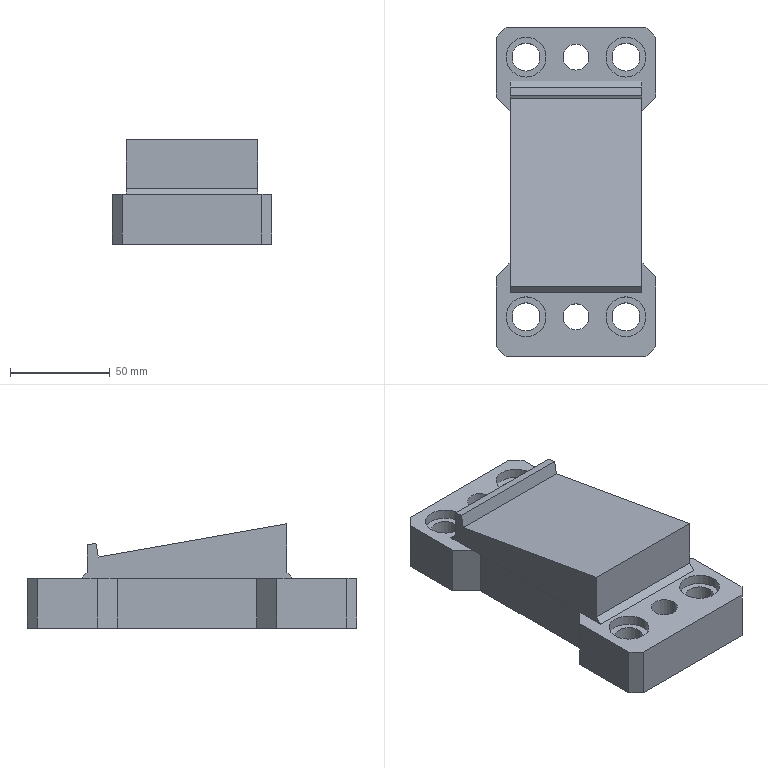Part | NX | features solid 2 | 1 solid | 45 faces | box 80 x 165 x 52.259 mm | volume 388189 mm3 | plane 31 | cylinder 10 | spline 4 | commonest cylinder face diameters 14 x4 20 x4 13 x2
STEP:
#1=CARTESIAN_POINT('',(-445.,-770.,-75.));
#2=VERTEX_POINT('',#1);
#3=CARTESIAN_POINT('',(-375.,-770.,-75.));
#4=VERTEX_POINT('',#3);
#5=CARTESIAN_POINT('',(-410.,-770.,-75.));
#6=DIRECTION('',(1.,0.,0.));
#7=VECTOR('',#6,1000.);
#8=LINE('',#5,#7);
#9=EDGE_CURVE('',#2,#4,#8,.T.);
#10=ORIENTED_EDGE('',*,*,#9,.T.);
#11=CARTESIAN_POINT('',(-370.,-765.,-75.));
#12=VERTEX_POINT('',#11);
#13=CARTESIAN_POINT('',(-351.25,-746.25,-75.));
#14=DIRECTION('',(0.7071,0.7071,0.));
#15=VECTOR('',#14,1000.);
#16=LINE('',#13,#15);
#17=EDGE_CURVE('',#12,#4,#16,.F.);
#18=ORIENTED_EDGE('',*,*,#17,.F.);
#19=CARTESIAN_POINT('',(-370.,-730.,-75.));
#20=VERTEX_POINT('',#19);
#21=CARTESIAN_POINT('',(-370.,-687.5,-75.));
#22=DIRECTION('',(0.,1.,0.));
#23=VECTOR('',#22,1000.);
#24=LINE('',#21,#23);
#25=EDGE_CURVE('',#12,#20,#24,.T.);
#26=ORIENTED_EDGE('',*,*,#25,.T.);
#27=CARTESIAN_POINT('',(-377.,-723.,-75.));
#28=VERTEX_POINT('',#27);
#29=CARTESIAN_POINT('',(-370.,-730.,-75.));
#30=DIRECTION('',(-0.7071,0.7071,0.));
#31=VECTOR('',#30,1000.);
#32=LINE('',#29,#31);
#33=EDGE_CURVE('',#20,#28,#32,.T.);
#34=ORIENTED_EDGE('',*,*,#33,.T.);
#35=CARTESIAN_POINT('',(-377.,-738.,-75.));
#36=VERTEX_POINT('',#35);
#37=CARTESIAN_POINT('',(-377.,-735.,-75.));
#38=DIRECTION('',(0.,1.,0.));
#39=VECTOR('',#38,1000.);
#40=LINE('',#37,#39);
#41=EDGE_CURVE('',#36,#28,#40,.T.);
#42=ORIENTED_EDGE('',*,*,#41,.F.);
#43=CARTESIAN_POINT('',(-443.,-738.,-75.));
#44=VERTEX_POINT('',#43);
#45=CARTESIAN_POINT('',(-410.,-738.,-75.));
#46=DIRECTION('',(1.,0.,0.));
#47=VECTOR('',#46,1000.);
#48=LINE('',#45,#47);
#49=EDGE_CURVE('',#44,#36,#48,.T.);
#50=ORIENTED_EDGE('',*,*,#49,.F.);
#51=CARTESIAN_POINT('',(-443.,-723.,-75.));
#52=VERTEX_POINT('',#51);
#53=CARTESIAN_POINT('',(-443.,-735.,-75.));
#54=DIRECTION('',(0.,1.,0.));
#55=VECTOR('',#54,1000.);
#56=LINE('',#53,#55);
#57=EDGE_CURVE('',#44,#52,#56,.T.);
#58=ORIENTED_EDGE('',*,*,#57,.T.);
#59=CARTESIAN_POINT('',(-450.,-730.,-75.));
#60=VERTEX_POINT('',#59);
#61=CARTESIAN_POINT('',(-440.,-720.,-75.));
#62=DIRECTION('',(-0.7071,-0.7071,0.));
#63=VECTOR('',#62,1000.);
#64=LINE('',#61,#63);
#65=EDGE_CURVE('',#52,#60,#64,.T.);
#66=ORIENTED_EDGE('',*,*,#65,.T.);
#67=CARTESIAN_POINT('',(-450.,-765.,-75.));
#68=VERTEX_POINT('',#67);
#69=CARTESIAN_POINT('',(-450.,-687.5,-75.));
#70=DIRECTION('',(0.,-1.,0.));
#71=VECTOR('',#70,1000.);
#72=LINE('',#69,#71);
#73=EDGE_CURVE('',#60,#68,#72,.T.);
#74=ORIENTED_EDGE('',*,*,#73,.T.);
#75=CARTESIAN_POINT('',(-468.75,-746.25,-75.));
#76=DIRECTION('',(0.7071,-0.7071,0.));
#77=VECTOR('',#76,1000.);
#78=LINE('',#75,#77);
#79=EDGE_CURVE('',#2,#68,#78,.F.);
#80=ORIENTED_EDGE('',*,*,#79,.F.);
#81=EDGE_LOOP('',(#10,#18,#26,#34,#42,#50,#58,#66,#74,#80));
#82=FACE_BOUND('',#81,.T.);
#83=CARTESIAN_POINT('',(-385.,-740.,-75.));
#84=VERTEX_POINT('',#83);
#85=CARTESIAN_POINT('',(-385.,-750.,-75.));
#86=DIRECTION('',(0.,0.,-1.));
#87=DIRECTION('',(0.,1.,0.));
#88=AXIS2_PLACEMENT_3D('',#85,#86,#87);
#89=CIRCLE('',#88,10.);
#90=EDGE_CURVE('',#84,#84,#89,.T.);
#91=ORIENTED_EDGE('',*,*,#90,.T.);
#92=EDGE_LOOP('',(#91));
#93=FACE_BOUND('',#92,.T.);
#94=CARTESIAN_POINT('',(-410.,-743.5,-75.));
#95=VERTEX_POINT('',#94);
#96=CARTESIAN_POINT('',(-410.,-750.,-75.));
#97=DIRECTION('',(0.,0.,-1.));
#98=DIRECTION('',(0.,1.,0.));
#99=AXIS2_PLACEMENT_3D('',#96,#97,#98);
#100=CIRCLE('',#99,6.5);
#101=EDGE_CURVE('',#95,#95,#100,.T.);
#102=ORIENTED_EDGE('',*,*,#101,.T.);
#103=EDGE_LOOP('',(#102));
#104=FACE_BOUND('',#103,.T.);
#105=CARTESIAN_POINT('',(-435.,-740.,-75.));
#106=VERTEX_POINT('',#105);
#107=CARTESIAN_POINT('',(-435.,-750.,-75.));
#108=DIRECTION('',(0.,0.,-1.));
#109=DIRECTION('',(0.,1.,0.));
#110=AXIS2_PLACEMENT_3D('',#107,#108,#109);
#111=CIRCLE('',#110,10.);
#112=EDGE_CURVE('',#106,#106,#111,.T.);
#113=ORIENTED_EDGE('',*,*,#112,.T.);
#114=EDGE_LOOP('',(#113));
#115=FACE_BOUND('',#114,.T.);
#116=CARTESIAN_POINT('',(-410.,-687.5,-75.));
#117=DIRECTION('',(0.,0.,1.));
#118=DIRECTION('',(0.,1.,0.));
#119=AXIS2_PLACEMENT_3D('',#116,#117,#118);
#120=PLANE('',#119);
#121=ADVANCED_FACE('',(#82,#93,#104,#115),#120,.T.);
#122=CARTESIAN_POINT('',(-375.,-605.,-75.));
#123=VERTEX_POINT('',#122);
#124=CARTESIAN_POINT('',(-445.,-605.,-75.));
#125=VERTEX_POINT('',#124);
#126=CARTESIAN_POINT('',(-410.,-605.,-75.));
#127=DIRECTION('',(-1.,0.,0.));
#128=VECTOR('',#127,1000.);
#129=LINE('',#126,#128);
#130=EDGE_CURVE('',#123,#125,#129,.T.);
#131=ORIENTED_EDGE('',*,*,#130,.T.);
#132=CARTESIAN_POINT('',(-450.,-610.,-75.));
#133=VERTEX_POINT('',#132);
#134=CARTESIAN_POINT('',(-468.75,-628.75,-75.));
#135=DIRECTION('',(-0.7071,-0.7071,0.));
#136=VECTOR('',#135,1000.);
#137=LINE('',#134,#136);
#138=EDGE_CURVE('',#133,#125,#137,.F.);
#139=ORIENTED_EDGE('',*,*,#138,.F.);
#140=CARTESIAN_POINT('',(-450.,-640.,-75.));
#141=VERTEX_POINT('',#140);
#142=CARTESIAN_POINT('',(-450.,-687.5,-75.));
#143=DIRECTION('',(0.,-1.,0.));
#144=VECTOR('',#143,1000.);
#145=LINE('',#142,#144);
#146=EDGE_CURVE('',#133,#141,#145,.T.);
#147=ORIENTED_EDGE('',*,*,#146,.T.);
#148=CARTESIAN_POINT('',(-443.,-647.,-75.));
#149=VERTEX_POINT('',#148);
#150=CARTESIAN_POINT('',(-440.,-650.,-75.));
#151=DIRECTION('',(-0.7071,0.7071,0.));
#152=VECTOR('',#151,1000.);
#153=LINE('',#150,#152);
#154=EDGE_CURVE('',#149,#141,#153,.T.);
#155=ORIENTED_EDGE('',*,*,#154,.F.);
#156=CARTESIAN_POINT('',(-443.,-632.,-75.));
#157=VERTEX_POINT('',#156);
#158=CARTESIAN_POINT('',(-443.,-735.,-75.));
#159=DIRECTION('',(0.,1.,0.));
#160=VECTOR('',#159,1000.);
#161=LINE('',#158,#160);
#162=EDGE_CURVE('',#149,#157,#161,.T.);
#163=ORIENTED_EDGE('',*,*,#162,.T.);
#164=CARTESIAN_POINT('',(-377.,-632.,-75.));
#165=VERTEX_POINT('',#164);
#166=CARTESIAN_POINT('',(-443.,-632.,-75.));
#167=DIRECTION('',(-1.,0.,0.));
#168=VECTOR('',#167,1000.);
#169=LINE('',#166,#168);
#170=EDGE_CURVE('',#165,#157,#169,.T.);
#171=ORIENTED_EDGE('',*,*,#170,.F.);
#172=CARTESIAN_POINT('',(-377.,-647.,-75.));
#173=VERTEX_POINT('',#172);
#174=CARTESIAN_POINT('',(-377.,-735.,-75.));
#175=DIRECTION('',(0.,1.,0.));
#176=VECTOR('',#175,1000.);
#177=LINE('',#174,#176);
#178=EDGE_CURVE('',#173,#165,#177,.T.);
#179=ORIENTED_EDGE('',*,*,#178,.F.);
#180=CARTESIAN_POINT('',(-370.,-640.,-75.));
#181=VERTEX_POINT('',#180);
#182=CARTESIAN_POINT('',(-370.,-640.,-75.));
#183=DIRECTION('',(-0.7071,-0.7071,0.));
#184=VECTOR('',#183,1000.);
#185=LINE('',#182,#184);
#186=EDGE_CURVE('',#181,#173,#185,.T.);
#187=ORIENTED_EDGE('',*,*,#186,.F.);
#188=CARTESIAN_POINT('',(-370.,-610.,-75.));
#189=VERTEX_POINT('',#188);
#190=CARTESIAN_POINT('',(-370.,-687.5,-75.));
#191=DIRECTION('',(0.,1.,0.));
#192=VECTOR('',#191,1000.);
#193=LINE('',#190,#192);
#194=EDGE_CURVE('',#181,#189,#193,.T.);
#195=ORIENTED_EDGE('',*,*,#194,.T.);
#196=CARTESIAN_POINT('',(-351.25,-628.75,-75.));
#197=DIRECTION('',(-0.7071,0.7071,0.));
#198=VECTOR('',#197,1000.);
#199=LINE('',#196,#198);
#200=EDGE_CURVE('',#123,#189,#199,.F.);
#201=ORIENTED_EDGE('',*,*,#200,.F.);
#202=EDGE_LOOP('',(#131,#139,#147,#155,#163,#171,#179,#187,#195,#201));
#203=FACE_BOUND('',#202,.T.);
#204=CARTESIAN_POINT('',(-385.,-610.,-75.));
#205=VERTEX_POINT('',#204);
#206=CARTESIAN_POINT('',(-385.,-620.,-75.));
#207=DIRECTION('',(0.,0.,-1.));
#208=DIRECTION('',(0.,1.,0.));
#209=AXIS2_PLACEMENT_3D('',#206,#207,#208);
#210=CIRCLE('',#209,10.);
#211=EDGE_CURVE('',#205,#205,#210,.T.);
#212=ORIENTED_EDGE('',*,*,#211,.T.);
#213=EDGE_LOOP('',(#212));
#214=FACE_BOUND('',#213,.T.);
#215=CARTESIAN_POINT('',(-410.,-613.5,-75.));
#216=VERTEX_POINT('',#215);
#217=CARTESIAN_POINT('',(-410.,-620.,-75.));
#218=DIRECTION('',(0.,0.,-1.));
#219=DIRECTION('',(0.,1.,0.));
#220=AXIS2_PLACEMENT_3D('',#217,#218,#219);
#221=CIRCLE('',#220,6.5);
#222=EDGE_CURVE('',#216,#216,#221,.T.);
#223=ORIENTED_EDGE('',*,*,#222,.T.);
#224=EDGE_LOOP('',(#223));
#225=FACE_BOUND('',#224,.T.);
#226=CARTESIAN_POINT('',(-435.,-610.,-75.));
#227=VERTEX_POINT('',#226);
#228=CARTESIAN_POINT('',(-435.,-620.,-75.));
#229=DIRECTION('',(0.,0.,-1.));
#230=DIRECTION('',(0.,1.,0.));
#231=AXIS2_PLACEMENT_3D('',#228,#229,#230);
#232=CIRCLE('',#231,10.);
#233=EDGE_CURVE('',#227,#227,#232,.T.);
#234=ORIENTED_EDGE('',*,*,#233,.T.);
#235=EDGE_LOOP('',(#234));
#236=FACE_BOUND('',#235,.T.);
#237=CARTESIAN_POINT('',(-410.,-687.5,-75.));
#238=DIRECTION('',(0.,0.,1.));
#239=DIRECTION('',(0.,1.,0.));
#240=AXIS2_PLACEMENT_3D('',#237,#238,#239);
#241=PLANE('',#240);
#242=ADVANCED_FACE('',(#203,#214,#225,#236),#241,.T.);
#243=CARTESIAN_POINT('',(-385.,-743.,-100.));
#244=VERTEX_POINT('',#243);
#245=CARTESIAN_POINT('',(-385.,-750.,-100.));
#246=DIRECTION('',(0.,0.,-1.));
#247=DIRECTION('',(0.,1.,0.));
#248=AXIS2_PLACEMENT_3D('',#245,#246,#247);
#249=CIRCLE('',#248,7.);
#250=EDGE_CURVE('',#244,#244,#249,.T.);
#251=ORIENTED_EDGE('',*,*,#250,.T.);
#252=EDGE_LOOP('',(#251));
#253=FACE_BOUND('',#252,.T.);
#254=CARTESIAN_POINT('',(-385.,-757.,-80.));
#255=VERTEX_POINT('',#254);
#256=CARTESIAN_POINT('',(-385.,-750.,-80.));
#257=DIRECTION('',(0.,0.,-1.));
#258=DIRECTION('',(0.,-1.,0.));
#259=AXIS2_PLACEMENT_3D('',#256,#257,#258);
#260=CIRCLE('',#259,7.);
#261=EDGE_CURVE('',#255,#255,#260,.T.);
#262=ORIENTED_EDGE('',*,*,#261,.F.);
#263=EDGE_LOOP('',(#262));
#264=FACE_BOUND('',#263,.T.);
#265=CARTESIAN_POINT('',(-385.,-750.,-75.));
#266=DIRECTION('',(0.,0.,-1.));
#267=DIRECTION('',(1.,0.,0.));
#268=AXIS2_PLACEMENT_3D('',#265,#266,#267);
#269=CYLINDRICAL_SURFACE('',#268,7.);
#270=ADVANCED_FACE('',(#253,#264),#269,.F.);
#271=CARTESIAN_POINT('',(-435.,-743.,-100.));
#272=VERTEX_POINT('',#271);
#273=CARTESIAN_POINT('',(-435.,-750.,-100.));
#274=DIRECTION('',(0.,0.,-1.));
#275=DIRECTION('',(0.,1.,0.));
#276=AXIS2_PLACEMENT_3D('',#273,#274,#275);
#277=CIRCLE('',#276,7.);
#278=EDGE_CURVE('',#272,#272,#277,.T.);
#279=ORIENTED_EDGE('',*,*,#278,.T.);
#280=EDGE_LOOP('',(#279));
#281=FACE_BOUND('',#280,.T.);
#282=CARTESIAN_POINT('',(-435.,-757.,-80.));
#283=VERTEX_POINT('',#282);
#284=CARTESIAN_POINT('',(-435.,-750.,-80.));
#285=DIRECTION('',(0.,0.,-1.));
#286=DIRECTION('',(0.,-1.,0.));
#287=AXIS2_PLACEMENT_3D('',#284,#285,#286);
#288=CIRCLE('',#287,7.);
#289=EDGE_CURVE('',#283,#283,#288,.T.);
#290=ORIENTED_EDGE('',*,*,#289,.F.);
#291=EDGE_LOOP('',(#290));
#292=FACE_BOUND('',#291,.T.);
#293=CARTESIAN_POINT('',(-435.,-750.,-75.));
#294=DIRECTION('',(0.,0.,-1.));
#295=DIRECTION('',(1.,0.,0.));
#296=AXIS2_PLACEMENT_3D('',#293,#294,#295);
#297=CYLINDRICAL_SURFACE('',#296,7.);
#298=ADVANCED_FACE('',(#281,#292),#297,.F.);
#299=CARTESIAN_POINT('',(-435.,-613.,-100.));
#300=VERTEX_POINT('',#299);
#301=CARTESIAN_POINT('',(-435.,-620.,-100.));
#302=DIRECTION('',(0.,0.,-1.));
#303=DIRECTION('',(0.,1.,0.));
#304=AXIS2_PLACEMENT_3D('',#301,#302,#303);
#305=CIRCLE('',#304,7.);
#306=EDGE_CURVE('',#300,#300,#305,.T.);
#307=ORIENTED_EDGE('',*,*,#306,.T.);
#308=EDGE_LOOP('',(#307));
#309=FACE_BOUND('',#308,.T.);
#310=CARTESIAN_POINT('',(-435.,-627.,-80.));
#311=VERTEX_POINT('',#310);
#312=CARTESIAN_POINT('',(-435.,-620.,-80.));
#313=DIRECTION('',(0.,0.,-1.));
#314=DIRECTION('',(0.,-1.,0.));
#315=AXIS2_PLACEMENT_3D('',#312,#313,#314);
#316=CIRCLE('',#315,7.);
#317=EDGE_CURVE('',#311,#311,#316,.T.);
#318=ORIENTED_EDGE('',*,*,#317,.F.);
#319=EDGE_LOOP('',(#318));
#320=FACE_BOUND('',#319,.T.);
#321=CARTESIAN_POINT('',(-435.,-620.,-75.));
#322=DIRECTION('',(0.,0.,-1.));
#323=DIRECTION('',(1.,0.,0.));
#324=AXIS2_PLACEMENT_3D('',#321,#322,#323);
#325=CYLINDRICAL_SURFACE('',#324,7.);
#326=ADVANCED_FACE('',(#309,#320),#325,.F.);
#327=CARTESIAN_POINT('',(-385.,-613.,-100.));
#328=VERTEX_POINT('',#327);
#329=CARTESIAN_POINT('',(-385.,-620.,-100.));
#330=DIRECTION('',(0.,0.,-1.));
#331=DIRECTION('',(0.,1.,0.));
#332=AXIS2_PLACEMENT_3D('',#329,#330,#331);
#333=CIRCLE('',#332,7.);
#334=EDGE_CURVE('',#328,#328,#333,.T.);
#335=ORIENTED_EDGE('',*,*,#334,.T.);
#336=EDGE_LOOP('',(#335));
#337=FACE_BOUND('',#336,.T.);
#338=CARTESIAN_POINT('',(-385.,-627.,-80.));
#339=VERTEX_POINT('',#338);
#340=CARTESIAN_POINT('',(-385.,-620.,-80.));
#341=DIRECTION('',(0.,0.,-1.));
#342=DIRECTION('',(0.,-1.,0.));
#343=AXIS2_PLACEMENT_3D('',#340,#341,#342);
#344=CIRCLE('',#343,7.);
#345=EDGE_CURVE('',#339,#339,#344,.T.);
#346=ORIENTED_EDGE('',*,*,#345,.F.);
#347=EDGE_LOOP('',(#346));
#348=FACE_BOUND('',#347,.T.);
#349=CARTESIAN_POINT('',(-385.,-620.,-75.));
#350=DIRECTION('',(0.,0.,-1.));
#351=DIRECTION('',(1.,0.,0.));
#352=AXIS2_PLACEMENT_3D('',#349,#350,#351);
#353=CYLINDRICAL_SURFACE('',#352,7.);
#354=ADVANCED_FACE('',(#337,#348),#353,.F.);
#355=CARTESIAN_POINT('',(-410.,-743.5,-100.));
#356=VERTEX_POINT('',#355);
#357=CARTESIAN_POINT('',(-410.,-750.,-100.));
#358=DIRECTION('',(0.,0.,-1.));
#359=DIRECTION('',(0.,1.,0.));
#360=AXIS2_PLACEMENT_3D('',#357,#358,#359);
#361=CIRCLE('',#360,6.5);
#362=EDGE_CURVE('',#356,#356,#361,.T.);
#363=ORIENTED_EDGE('',*,*,#362,.F.);
#364=EDGE_LOOP('',(#363));
#365=FACE_BOUND('',#364,.T.);
#366=ORIENTED_EDGE('',*,*,#306,.F.);
#367=EDGE_LOOP('',(#366));
#368=FACE_BOUND('',#367,.T.);
#369=ORIENTED_EDGE('',*,*,#334,.F.);
#370=EDGE_LOOP('',(#369));
#371=FACE_BOUND('',#370,.T.);
#372=CARTESIAN_POINT('',(-370.,-610.,-100.));
#373=VERTEX_POINT('',#372);
#374=CARTESIAN_POINT('',(-370.,-640.,-100.));
#375=VERTEX_POINT('',#374);
#376=CARTESIAN_POINT('',(-370.,-687.5,-100.));
#377=DIRECTION('',(0.,-1.,0.));
#378=VECTOR('',#377,1000.);
#379=LINE('',#376,#378);
#380=EDGE_CURVE('',#373,#375,#379,.T.);
#381=ORIENTED_EDGE('',*,*,#380,.T.);
#382=CARTESIAN_POINT('',(-380.,-650.,-100.));
#383=VERTEX_POINT('',#382);
#384=CARTESIAN_POINT('',(-370.,-640.,-100.));
#385=DIRECTION('',(-0.7071,-0.7071,0.));
#386=VECTOR('',#385,1000.);
#387=LINE('',#384,#386);
#388=EDGE_CURVE('',#375,#383,#387,.T.);
#389=ORIENTED_EDGE('',*,*,#388,.T.);
#390=CARTESIAN_POINT('',(-380.,-720.,-100.));
#391=VERTEX_POINT('',#390);
#392=CARTESIAN_POINT('',(-380.,-720.,-100.));
#393=DIRECTION('',(0.,1.,0.));
#394=VECTOR('',#393,1000.);
#395=LINE('',#392,#394);
#396=EDGE_CURVE('',#391,#383,#395,.T.);
#397=ORIENTED_EDGE('',*,*,#396,.F.);
#398=CARTESIAN_POINT('',(-370.,-730.,-100.));
#399=VERTEX_POINT('',#398);
#400=CARTESIAN_POINT('',(-370.,-730.,-100.));
#401=DIRECTION('',(-0.7071,0.7071,0.));
#402=VECTOR('',#401,1000.);
#403=LINE('',#400,#402);
#404=EDGE_CURVE('',#399,#391,#403,.T.);
#405=ORIENTED_EDGE('',*,*,#404,.F.);
#406=CARTESIAN_POINT('',(-370.,-765.,-100.));
#407=VERTEX_POINT('',#406);
#408=CARTESIAN_POINT('',(-370.,-687.5,-100.));
#409=DIRECTION('',(0.,-1.,0.));
#410=VECTOR('',#409,1000.);
#411=LINE('',#408,#410);
#412=EDGE_CURVE('',#399,#407,#411,.T.);
#413=ORIENTED_EDGE('',*,*,#412,.T.);
#414=CARTESIAN_POINT('',(-375.,-770.,-100.));
#415=VERTEX_POINT('',#414);
#416=CARTESIAN_POINT('',(-351.25,-746.25,-100.));
#417=DIRECTION('',(-0.7071,-0.7071,0.));
#418=VECTOR('',#417,1000.);
#419=LINE('',#416,#418);
#420=EDGE_CURVE('',#415,#407,#419,.F.);
#421=ORIENTED_EDGE('',*,*,#420,.F.);
#422=CARTESIAN_POINT('',(-445.,-770.,-100.));
#423=VERTEX_POINT('',#422);
#424=CARTESIAN_POINT('',(-410.,-770.,-100.));
#425=DIRECTION('',(-1.,0.,0.));
#426=VECTOR('',#425,1000.);
#427=LINE('',#424,#426);
#428=EDGE_CURVE('',#415,#423,#427,.T.);
#429=ORIENTED_EDGE('',*,*,#428,.T.);
#430=CARTESIAN_POINT('',(-450.,-765.,-100.));
#431=VERTEX_POINT('',#430);
#432=CARTESIAN_POINT('',(-468.75,-746.25,-100.));
#433=DIRECTION('',(-0.7071,0.7071,0.));
#434=VECTOR('',#433,1000.);
#435=LINE('',#432,#434);
#436=EDGE_CURVE('',#431,#423,#435,.F.);
#437=ORIENTED_EDGE('',*,*,#436,.F.);
#438=CARTESIAN_POINT('',(-450.,-730.,-100.));
#439=VERTEX_POINT('',#438);
#440=CARTESIAN_POINT('',(-450.,-687.5,-100.));
#441=DIRECTION('',(0.,1.,0.));
#442=VECTOR('',#441,1000.);
#443=LINE('',#440,#442);
#444=EDGE_CURVE('',#431,#439,#443,.T.);
#445=ORIENTED_EDGE('',*,*,#444,.T.);
#446=CARTESIAN_POINT('',(-440.,-720.,-100.));
#447=VERTEX_POINT('',#446);
#448=CARTESIAN_POINT('',(-440.,-720.,-100.));
#449=DIRECTION('',(-0.7071,-0.7071,0.));
#450=VECTOR('',#449,1000.);
#451=LINE('',#448,#450);
#452=EDGE_CURVE('',#447,#439,#451,.T.);
#453=ORIENTED_EDGE('',*,*,#452,.F.);
#454=CARTESIAN_POINT('',(-440.,-650.,-100.));
#455=VERTEX_POINT('',#454);
#456=CARTESIAN_POINT('',(-440.,-720.,-100.));
#457=DIRECTION('',(0.,1.,0.));
#458=VECTOR('',#457,1000.);
#459=LINE('',#456,#458);
#460=EDGE_CURVE('',#447,#455,#459,.T.);
#461=ORIENTED_EDGE('',*,*,#460,.T.);
#462=CARTESIAN_POINT('',(-450.,-640.,-100.));
#463=VERTEX_POINT('',#462);
#464=CARTESIAN_POINT('',(-440.,-650.,-100.));
#465=DIRECTION('',(-0.7071,0.7071,0.));
#466=VECTOR('',#465,1000.);
#467=LINE('',#464,#466);
#468=EDGE_CURVE('',#455,#463,#467,.T.);
#469=ORIENTED_EDGE('',*,*,#468,.T.);
#470=CARTESIAN_POINT('',(-450.,-610.,-100.));
#471=VERTEX_POINT('',#470);
#472=CARTESIAN_POINT('',(-450.,-687.5,-100.));
#473=DIRECTION('',(0.,1.,0.));
#474=VECTOR('',#473,1000.);
#475=LINE('',#472,#474);
#476=EDGE_CURVE('',#463,#471,#475,.T.);
#477=ORIENTED_EDGE('',*,*,#476,.T.);
#478=CARTESIAN_POINT('',(-445.,-605.,-100.));
#479=VERTEX_POINT('',#478);
#480=CARTESIAN_POINT('',(-468.75,-628.75,-100.));
#481=DIRECTION('',(0.7071,0.7071,0.));
#482=VECTOR('',#481,1000.);
#483=LINE('',#480,#482);
#484=EDGE_CURVE('',#479,#471,#483,.F.);
#485=ORIENTED_EDGE('',*,*,#484,.F.);
#486=CARTESIAN_POINT('',(-375.,-605.,-100.));
#487=VERTEX_POINT('',#486);
#488=CARTESIAN_POINT('',(-410.,-605.,-100.));
#489=DIRECTION('',(1.,0.,0.));
#490=VECTOR('',#489,1000.);
#491=LINE('',#488,#490);
#492=EDGE_CURVE('',#479,#487,#491,.T.);
#493=ORIENTED_EDGE('',*,*,#492,.T.);
#494=CARTESIAN_POINT('',(-351.25,-628.75,-100.));
#495=DIRECTION('',(0.7071,-0.7071,0.));
#496=VECTOR('',#495,1000.);
#497=LINE('',#494,#496);
#498=EDGE_CURVE('',#373,#487,#497,.F.);
#499=ORIENTED_EDGE('',*,*,#498,.F.);
#500=EDGE_LOOP('',(#381,#389,#397,#405,#413,#421,#429,#437,#445,#453,#461,#469,#477,#485,#493,#499));
#501=FACE_BOUND('',#500,.T.);
#502=CARTESIAN_POINT('',(-410.,-613.5,-100.));
#503=VERTEX_POINT('',#502);
#504=CARTESIAN_POINT('',(-410.,-620.,-100.));
#505=DIRECTION('',(0.,0.,-1.));
#506=DIRECTION('',(0.,1.,0.));
#507=AXIS2_PLACEMENT_3D('',#504,#505,#506);
#508=CIRCLE('',#507,6.5);
#509=EDGE_CURVE('',#503,#503,#508,.T.);
#510=ORIENTED_EDGE('',*,*,#509,.F.);
#511=EDGE_LOOP('',(#510));
#512=FACE_BOUND('',#511,.T.);
#513=ORIENTED_EDGE('',*,*,#250,.F.);
#514=EDGE_LOOP('',(#513));
#515=FACE_BOUND('',#514,.T.);
#516=ORIENTED_EDGE('',*,*,#278,.F.);
#517=EDGE_LOOP('',(#516));
#518=FACE_BOUND('',#517,.T.);
#519=CARTESIAN_POINT('',(-410.,-687.5,-100.));
#520=DIRECTION('',(0.,0.,-1.));
#521=DIRECTION('',(0.,-1.,0.));
#522=AXIS2_PLACEMENT_3D('',#519,#520,#521);
#523=PLANE('',#522);
#524=ADVANCED_FACE('',(#365,#368,#371,#501,#512,#515,#518),#523,.T.);
#525=ORIENTED_EDGE('',*,*,#73,.F.);
#526=CARTESIAN_POINT('',(-450.,-730.,-75.));
#527=DIRECTION('',(0.,0.,-1.));
#528=VECTOR('',#527,1000.);
#529=LINE('',#526,#528);
#530=EDGE_CURVE('',#60,#439,#529,.T.);
#531=ORIENTED_EDGE('',*,*,#530,.T.);
#532=ORIENTED_EDGE('',*,*,#444,.F.);
#533=CARTESIAN_POINT('',(-450.,-765.,-100.));
#534=DIRECTION('',(0.,0.,-1.));
#535=VECTOR('',#534,1000.);
#536=LINE('',#533,#535);
#537=EDGE_CURVE('',#68,#431,#536,.T.);
#538=ORIENTED_EDGE('',*,*,#537,.F.);
#539=EDGE_LOOP('',(#525,#531,#532,#538));
#540=FACE_BOUND('',#539,.T.);
#541=CARTESIAN_POINT('',(-450.,-687.5,-100.));
#542=DIRECTION('',(-1.,0.,0.));
#543=DIRECTION('',(0.,0.,-1.));
#544=AXIS2_PLACEMENT_3D('',#541,#542,#543);
#545=PLANE('',#544);
#546=ADVANCED_FACE('',(#540),#545,.T.);
#547=ORIENTED_EDGE('',*,*,#412,.F.);
#548=CARTESIAN_POINT('',(-370.,-730.,-75.));
#549=DIRECTION('',(0.,0.,-1.));
#550=VECTOR('',#549,1000.);
#551=LINE('',#548,#550);
#552=EDGE_CURVE('',#20,#399,#551,.T.);
#553=ORIENTED_EDGE('',*,*,#552,.F.);
#554=ORIENTED_EDGE('',*,*,#25,.F.);
#555=CARTESIAN_POINT('',(-370.,-765.,-100.));
#556=DIRECTION('',(0.,0.,1.));
#557=VECTOR('',#556,1000.);
#558=LINE('',#555,#557);
#559=EDGE_CURVE('',#407,#12,#558,.T.);
#560=ORIENTED_EDGE('',*,*,#559,.F.);
#561=EDGE_LOOP('',(#547,#553,#554,#560));
#562=FACE_BOUND('',#561,.T.);
#563=CARTESIAN_POINT('',(-370.,-687.5,-100.));
#564=DIRECTION('',(1.,0.,0.));
#565=DIRECTION('',(0.,0.,1.));
#566=AXIS2_PLACEMENT_3D('',#563,#564,#565);
#567=PLANE('',#566);
#568=ADVANCED_FACE('',(#562),#567,.T.);
#569=ORIENTED_EDGE('',*,*,#476,.F.);
#570=CARTESIAN_POINT('',(-450.,-640.,-75.));
#571=DIRECTION('',(0.,0.,-1.));
#572=VECTOR('',#571,1000.);
#573=LINE('',#570,#572);
#574=EDGE_CURVE('',#141,#463,#573,.T.);
#575=ORIENTED_EDGE('',*,*,#574,.F.);
#576=ORIENTED_EDGE('',*,*,#146,.F.);
#577=CARTESIAN_POINT('',(-450.,-610.,-100.));
#578=DIRECTION('',(0.,0.,1.));
#579=VECTOR('',#578,1000.);
#580=LINE('',#577,#579);
#581=EDGE_CURVE('',#471,#133,#580,.T.);
#582=ORIENTED_EDGE('',*,*,#581,.F.);
#583=EDGE_LOOP('',(#569,#575,#576,#582));
#584=FACE_BOUND('',#583,.T.);
#585=CARTESIAN_POINT('',(-450.,-687.5,-100.));
#586=DIRECTION('',(-1.,0.,0.));
#587=DIRECTION('',(0.,0.,-1.));
#588=AXIS2_PLACEMENT_3D('',#585,#586,#587);
#589=PLANE('',#588);
#590=ADVANCED_FACE('',(#584),#589,.T.);
#591=ORIENTED_EDGE('',*,*,#428,.F.);
#592=CARTESIAN_POINT('',(-375.,-770.,-100.));
#593=DIRECTION('',(0.,0.,-1.));
#594=VECTOR('',#593,1000.);
#595=LINE('',#592,#594);
#596=EDGE_CURVE('',#4,#415,#595,.T.);
#597=ORIENTED_EDGE('',*,*,#596,.F.);
#598=ORIENTED_EDGE('',*,*,#9,.F.);
#599=CARTESIAN_POINT('',(-445.,-770.,-100.));
#600=DIRECTION('',(0.,0.,1.));
#601=VECTOR('',#600,1000.);
#602=LINE('',#599,#601);
#603=EDGE_CURVE('',#423,#2,#602,.T.);
#604=ORIENTED_EDGE('',*,*,#603,.F.);
#605=EDGE_LOOP('',(#591,#597,#598,#604));
#606=FACE_BOUND('',#605,.T.);
#607=CARTESIAN_POINT('',(-410.,-770.,-100.));
#608=DIRECTION('',(0.,-1.,0.));
#609=DIRECTION('',(0.,0.,1.));
#610=AXIS2_PLACEMENT_3D('',#607,#608,#609);
#611=PLANE('',#610);
#612=ADVANCED_FACE('',(#606),#611,.T.);
#613=ORIENTED_EDGE('',*,*,#194,.F.);
#614=CARTESIAN_POINT('',(-370.,-640.,-75.));
#615=DIRECTION('',(0.,0.,-1.));
#616=VECTOR('',#615,1000.);
#617=LINE('',#614,#616);
#618=EDGE_CURVE('',#181,#375,#617,.T.);
#619=ORIENTED_EDGE('',*,*,#618,.T.);
#620=ORIENTED_EDGE('',*,*,#380,.F.);
#621=CARTESIAN_POINT('',(-370.,-610.,-100.));
#622=DIRECTION('',(0.,0.,-1.));
#623=VECTOR('',#622,1000.);
#624=LINE('',#621,#623);
#625=EDGE_CURVE('',#189,#373,#624,.T.);
#626=ORIENTED_EDGE('',*,*,#625,.F.);
#627=EDGE_LOOP('',(#613,#619,#620,#626));
#628=FACE_BOUND('',#627,.T.);
#629=CARTESIAN_POINT('',(-370.,-687.5,-100.));
#630=DIRECTION('',(1.,0.,0.));
#631=DIRECTION('',(0.,0.,1.));
#632=AXIS2_PLACEMENT_3D('',#629,#630,#631);
#633=PLANE('',#632);
#634=ADVANCED_FACE('',(#628),#633,.T.);
#635=ORIENTED_EDGE('',*,*,#492,.F.);
#636=CARTESIAN_POINT('',(-445.,-605.,-100.));
#637=DIRECTION('',(0.,0.,-1.));
#638=VECTOR('',#637,1000.);
#639=LINE('',#636,#638);
#640=EDGE_CURVE('',#125,#479,#639,.T.);
#641=ORIENTED_EDGE('',*,*,#640,.F.);
#642=ORIENTED_EDGE('',*,*,#130,.F.);
#643=CARTESIAN_POINT('',(-375.,-605.,-100.));
#644=DIRECTION('',(0.,0.,1.));
#645=VECTOR('',#644,1000.);
#646=LINE('',#643,#645);
#647=EDGE_CURVE('',#487,#123,#646,.T.);
#648=ORIENTED_EDGE('',*,*,#647,.F.);
#649=EDGE_LOOP('',(#635,#641,#642,#648));
#650=FACE_BOUND('',#649,.T.);
#651=CARTESIAN_POINT('',(-410.,-605.,-100.));
#652=DIRECTION('',(0.,1.,0.));
#653=DIRECTION('',(0.,0.,-1.));
#654=AXIS2_PLACEMENT_3D('',#651,#652,#653);
#655=PLANE('',#654);
#656=ADVANCED_FACE('',(#650),#655,.T.);
#657=ORIENTED_EDGE('',*,*,#388,.F.);
#658=ORIENTED_EDGE('',*,*,#618,.F.);
#659=ORIENTED_EDGE('',*,*,#186,.T.);
#660=CARTESIAN_POINT('',(-380.,-650.,-75.));
#661=VERTEX_POINT('',#660);
#662=CARTESIAN_POINT('',(-370.,-640.,-75.));
#663=DIRECTION('',(-0.7071,-0.7071,0.));
#664=VECTOR('',#663,1000.);
#665=LINE('',#662,#664);
#666=EDGE_CURVE('',#173,#661,#665,.T.);
#667=ORIENTED_EDGE('',*,*,#666,.T.);
#668=CARTESIAN_POINT('',(-380.,-650.,-75.));
#669=DIRECTION('',(0.,0.,-1.));
#670=VECTOR('',#669,1000.);
#671=LINE('',#668,#670);
#672=EDGE_CURVE('',#661,#383,#671,.T.);
#673=ORIENTED_EDGE('',*,*,#672,.T.);
#674=EDGE_LOOP('',(#657,#658,#659,#667,#673));
#675=FACE_BOUND('',#674,.T.);
#676=CARTESIAN_POINT('',(-370.,-640.,-75.));
#677=DIRECTION('',(-0.7071,0.7071,0.));
#678=DIRECTION('',(0.7071,0.7071,0.));
#679=AXIS2_PLACEMENT_3D('',#676,#677,#678);
#680=PLANE('',#679);
#681=ADVANCED_FACE('',(#675),#680,.F.);
#682=ORIENTED_EDGE('',*,*,#396,.T.);
#683=ORIENTED_EDGE('',*,*,#672,.F.);
#684=CARTESIAN_POINT('',(-380.,-720.,-75.));
#685=VERTEX_POINT('',#684);
#686=CARTESIAN_POINT('',(-380.,-720.,-75.));
#687=DIRECTION('',(0.,1.,0.));
#688=VECTOR('',#687,1000.);
#689=LINE('',#686,#688);
#690=EDGE_CURVE('',#685,#661,#689,.T.);
#691=ORIENTED_EDGE('',*,*,#690,.F.);
#692=CARTESIAN_POINT('',(-380.,-720.,-75.));
#693=DIRECTION('',(0.,0.,-1.));
#694=VECTOR('',#693,1000.);
#695=LINE('',#692,#694);
#696=EDGE_CURVE('',#685,#391,#695,.T.);
#697=ORIENTED_EDGE('',*,*,#696,.T.);
#698=EDGE_LOOP('',(#682,#683,#691,#697));
#699=FACE_BOUND('',#698,.T.);
#700=CARTESIAN_POINT('',(-380.,-720.,-75.));
#701=DIRECTION('',(1.,0.,0.));
#702=DIRECTION('',(0.,-1.,0.));
#703=AXIS2_PLACEMENT_3D('',#700,#701,#702);
#704=PLANE('',#703);
#705=ADVANCED_FACE('',(#699),#704,.T.);
#706=ORIENTED_EDGE('',*,*,#404,.T.);
#707=ORIENTED_EDGE('',*,*,#696,.F.);
#708=CARTESIAN_POINT('',(-370.,-730.,-75.));
#709=DIRECTION('',(-0.7071,0.7071,0.));
#710=VECTOR('',#709,1000.);
#711=LINE('',#708,#710);
#712=EDGE_CURVE('',#28,#685,#711,.T.);
#713=ORIENTED_EDGE('',*,*,#712,.F.);
#714=ORIENTED_EDGE('',*,*,#33,.F.);
#715=ORIENTED_EDGE('',*,*,#552,.T.);
#716=EDGE_LOOP('',(#706,#707,#713,#714,#715));
#717=FACE_BOUND('',#716,.T.);
#718=CARTESIAN_POINT('',(-370.,-730.,-75.));
#719=DIRECTION('',(0.7071,0.7071,0.));
#720=DIRECTION('',(0.7071,-0.7071,0.));
#721=AXIS2_PLACEMENT_3D('',#718,#719,#720);
#722=PLANE('',#721);
#723=ADVANCED_FACE('',(#717),#722,.T.);
#724=ORIENTED_EDGE('',*,*,#468,.F.);
#725=CARTESIAN_POINT('',(-440.,-650.,-75.));
#726=VERTEX_POINT('',#725);
#727=CARTESIAN_POINT('',(-440.,-650.,-75.));
#728=DIRECTION('',(0.,0.,-1.));
#729=VECTOR('',#728,1000.);
#730=LINE('',#727,#729);
#731=EDGE_CURVE('',#726,#455,#730,.T.);
#732=ORIENTED_EDGE('',*,*,#731,.F.);
#733=CARTESIAN_POINT('',(-440.,-650.,-75.));
#734=DIRECTION('',(-0.7071,0.7071,0.));
#735=VECTOR('',#734,1000.);
#736=LINE('',#733,#735);
#737=EDGE_CURVE('',#726,#149,#736,.T.);
#738=ORIENTED_EDGE('',*,*,#737,.T.);
#739=ORIENTED_EDGE('',*,*,#154,.T.);
#740=ORIENTED_EDGE('',*,*,#574,.T.);
#741=EDGE_LOOP('',(#724,#732,#738,#739,#740));
#742=FACE_BOUND('',#741,.T.);
#743=CARTESIAN_POINT('',(-440.,-650.,-75.));
#744=DIRECTION('',(0.7071,0.7071,0.));
#745=DIRECTION('',(0.7071,-0.7071,0.));
#746=AXIS2_PLACEMENT_3D('',#743,#744,#745);
#747=PLANE('',#746);
#748=ADVANCED_FACE('',(#742),#747,.F.);
#749=ORIENTED_EDGE('',*,*,#452,.T.);
#750=ORIENTED_EDGE('',*,*,#530,.F.);
#751=ORIENTED_EDGE('',*,*,#65,.F.);
#752=CARTESIAN_POINT('',(-440.,-720.,-75.));
#753=VERTEX_POINT('',#752);
#754=CARTESIAN_POINT('',(-440.,-720.,-75.));
#755=DIRECTION('',(-0.7071,-0.7071,0.));
#756=VECTOR('',#755,1000.);
#757=LINE('',#754,#756);
#758=EDGE_CURVE('',#753,#52,#757,.T.);
#759=ORIENTED_EDGE('',*,*,#758,.F.);
#760=CARTESIAN_POINT('',(-440.,-720.,-75.));
#761=DIRECTION('',(0.,0.,-1.));
#762=VECTOR('',#761,1000.);
#763=LINE('',#760,#762);
#764=EDGE_CURVE('',#753,#447,#763,.T.);
#765=ORIENTED_EDGE('',*,*,#764,.T.);
#766=EDGE_LOOP('',(#749,#750,#751,#759,#765));
#767=FACE_BOUND('',#766,.T.);
#768=CARTESIAN_POINT('',(-440.,-720.,-75.));
#769=DIRECTION('',(-0.7071,0.7071,0.));
#770=DIRECTION('',(0.7071,0.7071,0.));
#771=AXIS2_PLACEMENT_3D('',#768,#769,#770);
#772=PLANE('',#771);
#773=ADVANCED_FACE('',(#767),#772,.T.);
#774=ORIENTED_EDGE('',*,*,#460,.F.);
#775=ORIENTED_EDGE('',*,*,#764,.F.);
#776=CARTESIAN_POINT('',(-440.,-720.,-75.));
#777=DIRECTION('',(0.,1.,0.));
#778=VECTOR('',#777,1000.);
#779=LINE('',#776,#778);
#780=EDGE_CURVE('',#753,#726,#779,.T.);
#781=ORIENTED_EDGE('',*,*,#780,.T.);
#782=ORIENTED_EDGE('',*,*,#731,.T.);
#783=EDGE_LOOP('',(#774,#775,#781,#782));
#784=FACE_BOUND('',#783,.T.);
#785=CARTESIAN_POINT('',(-440.,-720.,-75.));
#786=DIRECTION('',(1.,0.,0.));
#787=DIRECTION('',(0.,-1.,0.));
#788=AXIS2_PLACEMENT_3D('',#785,#786,#787);
#789=PLANE('',#788);
#790=ADVANCED_FACE('',(#784),#789,.F.);
#791=ORIENTED_EDGE('',*,*,#222,.F.);
#792=EDGE_LOOP('',(#791));
#793=FACE_BOUND('',#792,.T.);
#794=ORIENTED_EDGE('',*,*,#509,.T.);
#795=EDGE_LOOP('',(#794));
#796=FACE_BOUND('',#795,.T.);
#797=CARTESIAN_POINT('',(-410.,-620.,-75.));
#798=DIRECTION('',(0.,0.,-1.));
#799=DIRECTION('',(1.,0.,0.));
#800=AXIS2_PLACEMENT_3D('',#797,#798,#799);
#801=CYLINDRICAL_SURFACE('',#800,6.5);
#802=ADVANCED_FACE('',(#793,#796),#801,.F.);
#803=ORIENTED_EDGE('',*,*,#101,.F.);
#804=EDGE_LOOP('',(#803));
#805=FACE_BOUND('',#804,.T.);
#806=ORIENTED_EDGE('',*,*,#362,.T.);
#807=EDGE_LOOP('',(#806));
#808=FACE_BOUND('',#807,.T.);
#809=CARTESIAN_POINT('',(-410.,-750.,-75.));
#810=DIRECTION('',(0.,0.,-1.));
#811=DIRECTION('',(1.,0.,0.));
#812=AXIS2_PLACEMENT_3D('',#809,#810,#811);
#813=CYLINDRICAL_SURFACE('',#812,6.5);
#814=ADVANCED_FACE('',(#805,#808),#813,.F.);
#815=ORIENTED_EDGE('',*,*,#211,.F.);
#816=EDGE_LOOP('',(#815));
#817=FACE_BOUND('',#816,.T.);
#818=CARTESIAN_POINT('',(-385.,-610.,-80.));
#819=VERTEX_POINT('',#818);
#820=CARTESIAN_POINT('',(-385.,-620.,-80.));
#821=DIRECTION('',(0.,0.,-1.));
#822=DIRECTION('',(0.,1.,0.));
#823=AXIS2_PLACEMENT_3D('',#820,#821,#822);
#824=CIRCLE('',#823,10.);
#825=EDGE_CURVE('',#819,#819,#824,.T.);
#826=ORIENTED_EDGE('',*,*,#825,.T.);
#827=EDGE_LOOP('',(#826));
#828=FACE_BOUND('',#827,.T.);
#829=CARTESIAN_POINT('',(-385.,-620.,-75.));
#830=DIRECTION('',(0.,0.,-1.));
#831=DIRECTION('',(1.,0.,0.));
#832=AXIS2_PLACEMENT_3D('',#829,#830,#831);
#833=CYLINDRICAL_SURFACE('',#832,10.);
#834=ADVANCED_FACE('',(#817,#828),#833,.F.);
#835=ORIENTED_EDGE('',*,*,#345,.T.);
#836=EDGE_LOOP('',(#835));
#837=FACE_BOUND('',#836,.T.);
#838=ORIENTED_EDGE('',*,*,#825,.F.);
#839=EDGE_LOOP('',(#838));
#840=FACE_BOUND('',#839,.T.);
#841=CARTESIAN_POINT('',(-385.,-620.,-80.));
#842=DIRECTION('',(0.,0.,1.));
#843=DIRECTION('',(0.,-1.,0.));
#844=AXIS2_PLACEMENT_3D('',#841,#842,#843);
#845=PLANE('',#844);
#846=ADVANCED_FACE('',(#837,#840),#845,.T.);
#847=ORIENTED_EDGE('',*,*,#233,.F.);
#848=EDGE_LOOP('',(#847));
#849=FACE_BOUND('',#848,.T.);
#850=CARTESIAN_POINT('',(-435.,-610.,-80.));
#851=VERTEX_POINT('',#850);
#852=CARTESIAN_POINT('',(-435.,-620.,-80.));
#853=DIRECTION('',(0.,0.,-1.));
#854=DIRECTION('',(0.,1.,0.));
#855=AXIS2_PLACEMENT_3D('',#852,#853,#854);
#856=CIRCLE('',#855,10.);
#857=EDGE_CURVE('',#851,#851,#856,.T.);
#858=ORIENTED_EDGE('',*,*,#857,.T.);
#859=EDGE_LOOP('',(#858));
#860=FACE_BOUND('',#859,.T.);
#861=CARTESIAN_POINT('',(-435.,-620.,-75.));
#862=DIRECTION('',(0.,0.,-1.));
#863=DIRECTION('',(1.,0.,0.));
#864=AXIS2_PLACEMENT_3D('',#861,#862,#863);
#865=CYLINDRICAL_SURFACE('',#864,10.);
#866=ADVANCED_FACE('',(#849,#860),#865,.F.);
#867=ORIENTED_EDGE('',*,*,#317,.T.);
#868=EDGE_LOOP('',(#867));
#869=FACE_BOUND('',#868,.T.);
#870=ORIENTED_EDGE('',*,*,#857,.F.);
#871=EDGE_LOOP('',(#870));
#872=FACE_BOUND('',#871,.T.);
#873=CARTESIAN_POINT('',(-435.,-620.,-80.));
#874=DIRECTION('',(0.,0.,1.));
#875=DIRECTION('',(0.,-1.,0.));
#876=AXIS2_PLACEMENT_3D('',#873,#874,#875);
#877=PLANE('',#876);
#878=ADVANCED_FACE('',(#869,#872),#877,.T.);
#879=ORIENTED_EDGE('',*,*,#112,.F.);
#880=EDGE_LOOP('',(#879));
#881=FACE_BOUND('',#880,.T.);
#882=CARTESIAN_POINT('',(-435.,-740.,-80.));
#883=VERTEX_POINT('',#882);
#884=CARTESIAN_POINT('',(-435.,-750.,-80.));
#885=DIRECTION('',(0.,0.,-1.));
#886=DIRECTION('',(0.,1.,0.));
#887=AXIS2_PLACEMENT_3D('',#884,#885,#886);
#888=CIRCLE('',#887,10.);
#889=EDGE_CURVE('',#883,#883,#888,.T.);
#890=ORIENTED_EDGE('',*,*,#889,.T.);
#891=EDGE_LOOP('',(#890));
#892=FACE_BOUND('',#891,.T.);
#893=CARTESIAN_POINT('',(-435.,-750.,-75.));
#894=DIRECTION('',(0.,0.,-1.));
#895=DIRECTION('',(1.,0.,0.));
#896=AXIS2_PLACEMENT_3D('',#893,#894,#895);
#897=CYLINDRICAL_SURFACE('',#896,10.);
#898=ADVANCED_FACE('',(#881,#892),#897,.F.);
#899=ORIENTED_EDGE('',*,*,#289,.T.);
#900=EDGE_LOOP('',(#899));
#901=FACE_BOUND('',#900,.T.);
#902=ORIENTED_EDGE('',*,*,#889,.F.);
#903=EDGE_LOOP('',(#902));
#904=FACE_BOUND('',#903,.T.);
#905=CARTESIAN_POINT('',(-435.,-750.,-80.));
#906=DIRECTION('',(0.,0.,1.));
#907=DIRECTION('',(0.,-1.,0.));
#908=AXIS2_PLACEMENT_3D('',#905,#906,#907);
#909=PLANE('',#908);
#910=ADVANCED_FACE('',(#901,#904),#909,.T.);
#911=ORIENTED_EDGE('',*,*,#90,.F.);
#912=EDGE_LOOP('',(#911));
#913=FACE_BOUND('',#912,.T.);
#914=CARTESIAN_POINT('',(-385.,-740.,-80.));
#915=VERTEX_POINT('',#914);
#916=CARTESIAN_POINT('',(-385.,-750.,-80.));
#917=DIRECTION('',(0.,0.,-1.));
#918=DIRECTION('',(0.,1.,0.));
#919=AXIS2_PLACEMENT_3D('',#916,#917,#918);
#920=CIRCLE('',#919,10.);
#921=EDGE_CURVE('',#915,#915,#920,.T.);
#922=ORIENTED_EDGE('',*,*,#921,.T.);
#923=EDGE_LOOP('',(#922));
#924=FACE_BOUND('',#923,.T.);
#925=CARTESIAN_POINT('',(-385.,-750.,-75.));
#926=DIRECTION('',(0.,0.,-1.));
#927=DIRECTION('',(1.,0.,0.));
#928=AXIS2_PLACEMENT_3D('',#925,#926,#927);
#929=CYLINDRICAL_SURFACE('',#928,10.);
#930=ADVANCED_FACE('',(#913,#924),#929,.F.);
#931=ORIENTED_EDGE('',*,*,#261,.T.);
#932=EDGE_LOOP('',(#931));
#933=FACE_BOUND('',#932,.T.);
#934=ORIENTED_EDGE('',*,*,#921,.F.);
#935=EDGE_LOOP('',(#934));
#936=FACE_BOUND('',#935,.T.);
#937=CARTESIAN_POINT('',(-385.,-750.,-80.));
#938=DIRECTION('',(0.,0.,1.));
#939=DIRECTION('',(0.,-1.,0.));
#940=AXIS2_PLACEMENT_3D('',#937,#938,#939);
#941=PLANE('',#940);
#942=ADVANCED_FACE('',(#933,#936),#941,.T.);
#943=ORIENTED_EDGE('',*,*,#758,.T.);
#944=CARTESIAN_POINT('',(-443.,-735.,-75.));
#945=DIRECTION('',(0.,1.,0.));
#946=VECTOR('',#945,1000.);
#947=LINE('',#944,#946);
#948=EDGE_CURVE('',#52,#149,#947,.T.);
#949=ORIENTED_EDGE('',*,*,#948,.T.);
#950=ORIENTED_EDGE('',*,*,#737,.F.);
#951=ORIENTED_EDGE('',*,*,#780,.F.);
#952=EDGE_LOOP('',(#943,#949,#950,#951));
#953=FACE_BOUND('',#952,.T.);
#954=CARTESIAN_POINT('',(-377.,-735.,-75.));
#955=DIRECTION('',(0.,0.,-1.));
#956=DIRECTION('',(1.,0.,0.));
#957=AXIS2_PLACEMENT_3D('',#954,#955,#956);
#958=PLANE('',#957);
#959=ADVANCED_FACE('',(#953),#958,.T.);
#960=CARTESIAN_POINT('',(-377.,-735.,-72.));
#961=VERTEX_POINT('',#960);
#962=CARTESIAN_POINT('',(-377.,-735.,-47.741));
#963=VERTEX_POINT('',#962);
#964=CARTESIAN_POINT('',(-377.,-735.,-75.));
#965=DIRECTION('',(0.,0.,1.));
#966=VECTOR('',#965,1000.);
#967=LINE('',#964,#966);
#968=EDGE_CURVE('',#961,#963,#967,.T.);
#969=ORIENTED_EDGE('',*,*,#968,.T.);
#970=CARTESIAN_POINT('',(-443.,-735.,-47.741));
#971=VERTEX_POINT('',#970);
#972=CARTESIAN_POINT('',(-377.,-735.,-47.741));
#973=DIRECTION('',(-1.,0.,0.));
#974=VECTOR('',#973,1000.);
#975=LINE('',#972,#974);
#976=EDGE_CURVE('',#963,#971,#975,.T.);
#977=ORIENTED_EDGE('',*,*,#976,.T.);
#978=CARTESIAN_POINT('',(-443.,-735.,-72.));
#979=VERTEX_POINT('',#978);
#980=CARTESIAN_POINT('',(-443.,-735.,-75.));
#981=DIRECTION('',(0.,0.,1.));
#982=VECTOR('',#981,1000.);
#983=LINE('',#980,#982);
#984=EDGE_CURVE('',#979,#971,#983,.T.);
#985=ORIENTED_EDGE('',*,*,#984,.F.);
#986=CARTESIAN_POINT('',(-377.,-735.,-72.));
#987=DIRECTION('',(-1.,0.,0.));
#988=VECTOR('',#987,1000.);
#989=LINE('',#986,#988);
#990=EDGE_CURVE('',#961,#979,#989,.T.);
#991=ORIENTED_EDGE('',*,*,#990,.F.);
#992=EDGE_LOOP('',(#969,#977,#985,#991));
#993=FACE_BOUND('',#992,.T.);
#994=CARTESIAN_POINT('',(-377.,-735.,-75.));
#995=DIRECTION('',(0.,1.,0.));
#996=DIRECTION('',(1.,0.,0.));
#997=AXIS2_PLACEMENT_3D('',#994,#995,#996);
#998=PLANE('',#997);
#999=ADVANCED_FACE('',(#993),#998,.F.);
#1000=ORIENTED_EDGE('',*,*,#41,.T.);
#1001=CARTESIAN_POINT('',(-377.,-735.,-75.));
#1002=DIRECTION('',(0.,1.,0.));
#1003=VECTOR('',#1002,1000.);
#1004=LINE('',#1001,#1003);
#1005=EDGE_CURVE('',#28,#173,#1004,.T.);
#1006=ORIENTED_EDGE('',*,*,#1005,.T.);
#1007=ORIENTED_EDGE('',*,*,#178,.T.);
#1008=CARTESIAN_POINT('',(-377.,-635.,-72.));
#1009=VERTEX_POINT('',#1008);
#1010=CARTESIAN_POINT('',(-377.,-632.,-75.));
#1011=DIRECTION('',(0.,-0.7071,0.7071));
#1012=VECTOR('',#1011,1000.);
#1013=LINE('',#1010,#1012);
#1014=EDGE_CURVE('',#1009,#165,#1013,.F.);
#1015=ORIENTED_EDGE('',*,*,#1014,.F.);
#1016=CARTESIAN_POINT('',(-377.,-635.,-58.273));
#1017=VERTEX_POINT('',#1016);
#1018=CARTESIAN_POINT('',(-377.,-635.,-75.));
#1019=DIRECTION('',(0.,0.,1.));
#1020=VECTOR('',#1019,1000.);
#1021=LINE('',#1018,#1020);
#1022=EDGE_CURVE('',#1009,#1017,#1021,.T.);
#1023=ORIENTED_EDGE('',*,*,#1022,.T.);
#1024=CARTESIAN_POINT('',(-377.,-635.039,-58.259));
#1025=VERTEX_POINT('',#1024);
#1026=CARTESIAN_POINT('',(-377.,-630.011,-60.089));
#1027=CARTESIAN_POINT('',(-377.,-641.282,-55.986));
#1028=B_SPLINE_CURVE_WITH_KNOTS('',1,(#1026,#1027),.UNSPECIFIED.,.F.,.F.,(2,2),(0.,1.),.PIECEWISE_BEZIER_KNOTS.);
#1029=EDGE_CURVE('',#1017,#1025,#1028,.T.);
#1030=ORIENTED_EDGE('',*,*,#1029,.T.);
#1031=CARTESIAN_POINT('',(-377.,-639.417,-57.487));
#1032=VERTEX_POINT('',#1031);
#1033=CARTESIAN_POINT('',(-377.,-626.249,-59.809));
#1034=CARTESIAN_POINT('',(-377.,-639.417,-57.487));
#1035=B_SPLINE_CURVE_WITH_KNOTS('',1,(#1033,#1034),.UNSPECIFIED.,.F.,.F.,(2,2),(0.,1.),.PIECEWISE_BEZIER_KNOTS.);
#1036=EDGE_CURVE('',#1025,#1032,#1035,.T.);
#1037=ORIENTED_EDGE('',*,*,#1036,.T.);
#1038=CARTESIAN_POINT('',(-377.,-640.633,-64.38));
#1039=VERTEX_POINT('',#1038);
#1040=CARTESIAN_POINT('',(-377.,-639.417,-57.487));
#1041=CARTESIAN_POINT('',(-377.,-640.633,-64.38));
#1042=B_SPLINE_CURVE_WITH_KNOTS('',1,(#1040,#1041),.UNSPECIFIED.,.F.,.F.,(2,2),(0.,1.),.PIECEWISE_BEZIER_KNOTS.);
#1043=EDGE_CURVE('',#1032,#1039,#1042,.T.);
#1044=ORIENTED_EDGE('',*,*,#1043,.T.);
#1045=CARTESIAN_POINT('',(-377.,-640.633,-64.38));
#1046=CARTESIAN_POINT('',(-377.,-755.691,-44.092));
#1047=B_SPLINE_CURVE_WITH_KNOTS('',1,(#1045,#1046),.UNSPECIFIED.,.F.,.F.,(2,2),(0.,1.),.PIECEWISE_BEZIER_KNOTS.);
#1048=EDGE_CURVE('',#1039,#963,#1047,.T.);
#1049=ORIENTED_EDGE('',*,*,#1048,.T.);
#1050=ORIENTED_EDGE('',*,*,#968,.F.);
#1051=CARTESIAN_POINT('',(-377.,-735.,-72.));
#1052=DIRECTION('',(0.,0.7071,0.7071));
#1053=VECTOR('',#1052,1000.);
#1054=LINE('',#1051,#1053);
#1055=EDGE_CURVE('',#36,#961,#1054,.T.);
#1056=ORIENTED_EDGE('',*,*,#1055,.F.);
#1057=EDGE_LOOP('',(#1000,#1006,#1007,#1015,#1023,#1030,#1037,#1044,#1049,#1050,#1056));
#1058=FACE_BOUND('',#1057,.T.);
#1059=CARTESIAN_POINT('',(-377.,-735.,-8.254));
#1060=DIRECTION('',(1.,0.,0.));
#1061=DIRECTION('',(0.,-1.,0.));
#1062=AXIS2_PLACEMENT_3D('',#1059,#1060,#1061);
#1063=PLANE('',#1062);
#1064=ADVANCED_FACE('',(#1058),#1063,.T.);
#1065=CARTESIAN_POINT('',(-443.,-640.633,-64.38));
#1066=VERTEX_POINT('',#1065);
#1067=CARTESIAN_POINT('',(-443.,-640.633,-64.38));
#1068=CARTESIAN_POINT('',(-443.,-755.691,-44.092));
#1069=B_SPLINE_CURVE_WITH_KNOTS('',1,(#1067,#1068),.UNSPECIFIED.,.F.,.F.,(2,2),(0.,1.),.PIECEWISE_BEZIER_KNOTS.);
#1070=EDGE_CURVE('',#971,#1066,#1069,.F.);
#1071=ORIENTED_EDGE('',*,*,#1070,.T.);
#1072=CARTESIAN_POINT('',(-443.,-639.417,-57.487));
#1073=VERTEX_POINT('',#1072);
#1074=CARTESIAN_POINT('',(-443.,-639.417,-57.487));
#1075=CARTESIAN_POINT('',(-443.,-640.633,-64.38));
#1076=B_SPLINE_CURVE_WITH_KNOTS('',1,(#1074,#1075),.UNSPECIFIED.,.F.,.F.,(2,2),(0.,1.),.PIECEWISE_BEZIER_KNOTS.);
#1077=EDGE_CURVE('',#1066,#1073,#1076,.F.);
#1078=ORIENTED_EDGE('',*,*,#1077,.T.);
#1079=CARTESIAN_POINT('',(-443.,-635.039,-58.259));
#1080=VERTEX_POINT('',#1079);
#1081=CARTESIAN_POINT('',(-443.,-626.249,-59.809));
#1082=CARTESIAN_POINT('',(-443.,-639.417,-57.487));
#1083=B_SPLINE_CURVE_WITH_KNOTS('',1,(#1081,#1082),.UNSPECIFIED.,.F.,.F.,(2,2),(0.,1.),.PIECEWISE_BEZIER_KNOTS.);
#1084=EDGE_CURVE('',#1073,#1080,#1083,.F.);
#1085=ORIENTED_EDGE('',*,*,#1084,.T.);
#1086=CARTESIAN_POINT('',(-443.,-635.,-58.273));
#1087=VERTEX_POINT('',#1086);
#1088=CARTESIAN_POINT('',(-443.,-630.011,-60.089));
#1089=CARTESIAN_POINT('',(-443.,-641.282,-55.986));
#1090=B_SPLINE_CURVE_WITH_KNOTS('',1,(#1088,#1089),.UNSPECIFIED.,.F.,.F.,(2,2),(0.,1.),.PIECEWISE_BEZIER_KNOTS.);
#1091=EDGE_CURVE('',#1080,#1087,#1090,.F.);
#1092=ORIENTED_EDGE('',*,*,#1091,.T.);
#1093=CARTESIAN_POINT('',(-443.,-635.,-72.));
#1094=VERTEX_POINT('',#1093);
#1095=CARTESIAN_POINT('',(-443.,-635.,-75.));
#1096=DIRECTION('',(0.,0.,1.));
#1097=VECTOR('',#1096,1000.);
#1098=LINE('',#1095,#1097);
#1099=EDGE_CURVE('',#1094,#1087,#1098,.T.);
#1100=ORIENTED_EDGE('',*,*,#1099,.F.);
#1101=CARTESIAN_POINT('',(-443.,-716.873,9.873));
#1102=DIRECTION('',(0.,0.7071,-0.7071));
#1103=VECTOR('',#1102,1000.);
#1104=LINE('',#1101,#1103);
#1105=EDGE_CURVE('',#157,#1094,#1104,.F.);
#1106=ORIENTED_EDGE('',*,*,#1105,.F.);
#1107=ORIENTED_EDGE('',*,*,#162,.F.);
#1108=ORIENTED_EDGE('',*,*,#948,.F.);
#1109=ORIENTED_EDGE('',*,*,#57,.F.);
#1110=CARTESIAN_POINT('',(-443.,-703.127,-40.127));
#1111=DIRECTION('',(0.,-0.7071,-0.7071));
#1112=VECTOR('',#1111,1000.);
#1113=LINE('',#1110,#1112);
#1114=EDGE_CURVE('',#979,#44,#1113,.T.);
#1115=ORIENTED_EDGE('',*,*,#1114,.F.);
#1116=ORIENTED_EDGE('',*,*,#984,.T.);
#1117=EDGE_LOOP('',(#1071,#1078,#1085,#1092,#1100,#1106,#1107,#1108,#1109,#1115,#1116));
#1118=FACE_BOUND('',#1117,.T.);
#1119=CARTESIAN_POINT('',(-443.,-735.,-8.254));
#1120=DIRECTION('',(1.,0.,0.));
#1121=DIRECTION('',(0.,-1.,0.));
#1122=AXIS2_PLACEMENT_3D('',#1119,#1120,#1121);
#1123=PLANE('',#1122);
#1124=ADVANCED_FACE('',(#1118),#1123,.F.);
#1125=ORIENTED_EDGE('',*,*,#1029,.F.);
#1126=CARTESIAN_POINT('',(-377.,-635.,-58.273));
#1127=DIRECTION('',(-1.,0.,0.));
#1128=VECTOR('',#1127,1000.);
#1129=LINE('',#1126,#1128);
#1130=EDGE_CURVE('',#1017,#1087,#1129,.T.);
#1131=ORIENTED_EDGE('',*,*,#1130,.T.);
#1132=ORIENTED_EDGE('',*,*,#1091,.F.);
#1133=CARTESIAN_POINT('',(-410.,-635.039,-58.259));
#1134=DIRECTION('',(-1.,0.,0.));
#1135=VECTOR('',#1134,1000.);
#1136=LINE('',#1133,#1135);
#1137=EDGE_CURVE('',#1025,#1080,#1136,.T.);
#1138=ORIENTED_EDGE('',*,*,#1137,.F.);
#1139=EDGE_LOOP('',(#1125,#1131,#1132,#1138));
#1140=FACE_BOUND('',#1139,.T.);
#1141=CARTESIAN_POINT('',(-377.,-635.,-58.273));
#1142=CARTESIAN_POINT('',(-443.,-635.,-58.273));
#1143=CARTESIAN_POINT('',(-377.,-635.039,-58.259));
#1144=CARTESIAN_POINT('',(-443.,-635.039,-58.259));
#1145=B_SPLINE_SURFACE_WITH_KNOTS('',1,1,((#1141,#1142),(#1143,#1144)),.SURF_OF_LINEAR_EXTRUSION.,.F.,.F.,.F.,(2,2),(2,2),(0.4426,0.4461),(0.,1.),.PIECEWISE_BEZIER_KNOTS.);
#1146=ADVANCED_FACE('',(#1140),#1145,.F.);
#1147=ORIENTED_EDGE('',*,*,#1099,.T.);
#1148=ORIENTED_EDGE('',*,*,#1130,.F.);
#1149=ORIENTED_EDGE('',*,*,#1022,.F.);
#1150=CARTESIAN_POINT('',(-377.,-635.,-72.));
#1151=DIRECTION('',(1.,0.,0.));
#1152=VECTOR('',#1151,1000.);
#1153=LINE('',#1150,#1152);
#1154=EDGE_CURVE('',#1094,#1009,#1153,.T.);
#1155=ORIENTED_EDGE('',*,*,#1154,.F.);
#1156=EDGE_LOOP('',(#1147,#1148,#1149,#1155));
#1157=FACE_BOUND('',#1156,.T.);
#1158=CARTESIAN_POINT('',(-377.,-635.,-75.));
#1159=DIRECTION('',(0.,1.,0.));
#1160=DIRECTION('',(1.,0.,0.));
#1161=AXIS2_PLACEMENT_3D('',#1158,#1159,#1160);
#1162=PLANE('',#1161);
#1163=ADVANCED_FACE('',(#1157),#1162,.T.);
#1164=ORIENTED_EDGE('',*,*,#1005,.F.);
#1165=ORIENTED_EDGE('',*,*,#712,.T.);
#1166=ORIENTED_EDGE('',*,*,#690,.T.);
#1167=ORIENTED_EDGE('',*,*,#666,.F.);
#1168=EDGE_LOOP('',(#1164,#1165,#1166,#1167));
#1169=FACE_BOUND('',#1168,.T.);
#1170=CARTESIAN_POINT('',(-377.,-735.,-75.));
#1171=DIRECTION('',(0.,0.,-1.));
#1172=DIRECTION('',(1.,0.,0.));
#1173=AXIS2_PLACEMENT_3D('',#1170,#1171,#1172);
#1174=PLANE('',#1173);
#1175=ADVANCED_FACE('',(#1169),#1174,.T.);
#1176=ORIENTED_EDGE('',*,*,#1048,.F.);
#1177=CARTESIAN_POINT('',(-377.,-640.633,-64.38));
#1178=CARTESIAN_POINT('',(-443.,-640.633,-64.38));
#1179=B_SPLINE_CURVE_WITH_KNOTS('',1,(#1177,#1178),.UNSPECIFIED.,.F.,.F.,(2,2),(0.,1.),.PIECEWISE_BEZIER_KNOTS.);
#1180=EDGE_CURVE('',#1066,#1039,#1179,.F.);
#1181=ORIENTED_EDGE('',*,*,#1180,.F.);
#1182=ORIENTED_EDGE('',*,*,#1070,.F.);
#1183=ORIENTED_EDGE('',*,*,#976,.F.);
#1184=EDGE_LOOP('',(#1176,#1181,#1182,#1183));
#1185=FACE_BOUND('',#1184,.T.);
#1186=CARTESIAN_POINT('',(-377.,-640.633,-64.38));
#1187=CARTESIAN_POINT('',(-443.,-640.633,-64.38));
#1188=CARTESIAN_POINT('',(-377.,-735.,-47.741));
#1189=CARTESIAN_POINT('',(-443.,-735.,-47.741));
#1190=B_SPLINE_SURFACE_WITH_KNOTS('',1,1,((#1186,#1187),(#1188,#1189)),.SURF_OF_LINEAR_EXTRUSION.,.F.,.F.,.F.,(2,2),(2,2),(0.,0.8202),(0.,1.),.PIECEWISE_BEZIER_KNOTS.);
#1191=ADVANCED_FACE('',(#1185),#1190,.F.);
#1192=ORIENTED_EDGE('',*,*,#1043,.F.);
#1193=CARTESIAN_POINT('',(-377.,-639.417,-57.487));
#1194=CARTESIAN_POINT('',(-443.,-639.417,-57.487));
#1195=B_SPLINE_CURVE_WITH_KNOTS('',1,(#1193,#1194),.UNSPECIFIED.,.F.,.F.,(2,2),(0.,1.),.PIECEWISE_BEZIER_KNOTS.);
#1196=EDGE_CURVE('',#1073,#1032,#1195,.F.);
#1197=ORIENTED_EDGE('',*,*,#1196,.F.);
#1198=ORIENTED_EDGE('',*,*,#1077,.F.);
#1199=ORIENTED_EDGE('',*,*,#1180,.T.);
#1200=EDGE_LOOP('',(#1192,#1197,#1198,#1199));
#1201=FACE_BOUND('',#1200,.T.);
#1202=CARTESIAN_POINT('',(-377.,-639.417,-57.487));
#1203=CARTESIAN_POINT('',(-443.,-639.417,-57.487));
#1204=CARTESIAN_POINT('',(-377.,-640.633,-64.38));
#1205=CARTESIAN_POINT('',(-443.,-640.633,-64.38));
#1206=B_SPLINE_SURFACE_WITH_KNOTS('',1,1,((#1202,#1203),(#1204,#1205)),.SURF_OF_LINEAR_EXTRUSION.,.F.,.F.,.F.,(2,2),(2,2),(0.,1.),(0.,1.),.PIECEWISE_BEZIER_KNOTS.);
#1207=ADVANCED_FACE('',(#1201),#1206,.F.);
#1208=ORIENTED_EDGE('',*,*,#1137,.T.);
#1209=ORIENTED_EDGE('',*,*,#1084,.F.);
#1210=ORIENTED_EDGE('',*,*,#1196,.T.);
#1211=ORIENTED_EDGE('',*,*,#1036,.F.);
#1212=EDGE_LOOP('',(#1208,#1209,#1210,#1211));
#1213=FACE_BOUND('',#1212,.T.);
#1214=CARTESIAN_POINT('',(-377.,-635.039,-58.259));
#1215=CARTESIAN_POINT('',(-443.,-635.039,-58.259));
#1216=CARTESIAN_POINT('',(-377.,-639.417,-57.487));
#1217=CARTESIAN_POINT('',(-443.,-639.417,-57.487));
#1218=B_SPLINE_SURFACE_WITH_KNOTS('',1,1,((#1214,#1215),(#1216,#1217)),.SURF_OF_LINEAR_EXTRUSION.,.F.,.F.,.F.,(2,2),(2,2),(0.6675,1.),(0.,1.),.PIECEWISE_BEZIER_KNOTS.);
#1219=ADVANCED_FACE('',(#1213),#1218,.F.);
#1220=ORIENTED_EDGE('',*,*,#1055,.T.);
#1221=ORIENTED_EDGE('',*,*,#990,.T.);
#1222=ORIENTED_EDGE('',*,*,#1114,.T.);
#1223=ORIENTED_EDGE('',*,*,#49,.T.);
#1224=EDGE_LOOP('',(#1220,#1221,#1222,#1223));
#1225=FACE_BOUND('',#1224,.T.);
#1226=CARTESIAN_POINT('',(-377.,-735.,-72.));
#1227=DIRECTION('',(0.,0.7071,-0.7071));
#1228=DIRECTION('',(0.,0.7071,0.7071));
#1229=AXIS2_PLACEMENT_3D('',#1226,#1227,#1228);
#1230=PLANE('',#1229);
#1231=ADVANCED_FACE('',(#1225),#1230,.F.);
#1232=ORIENTED_EDGE('',*,*,#1014,.T.);
#1233=ORIENTED_EDGE('',*,*,#170,.T.);
#1234=ORIENTED_EDGE('',*,*,#1105,.T.);
#1235=ORIENTED_EDGE('',*,*,#1154,.T.);
#1236=EDGE_LOOP('',(#1232,#1233,#1234,#1235));
#1237=FACE_BOUND('',#1236,.T.);
#1238=CARTESIAN_POINT('',(-410.,-632.,-75.));
#1239=DIRECTION('',(0.,0.7071,0.7071));
#1240=DIRECTION('',(0.,-0.7071,0.7071));
#1241=AXIS2_PLACEMENT_3D('',#1238,#1239,#1240);
#1242=PLANE('',#1241);
#1243=ADVANCED_FACE('',(#1237),#1242,.T.);
#1244=ORIENTED_EDGE('',*,*,#200,.T.);
#1245=ORIENTED_EDGE('',*,*,#625,.T.);
#1246=ORIENTED_EDGE('',*,*,#498,.T.);
#1247=ORIENTED_EDGE('',*,*,#647,.T.);
#1248=EDGE_LOOP('',(#1244,#1245,#1246,#1247));
#1249=FACE_BOUND('',#1248,.T.);
#1250=CARTESIAN_POINT('',(-370.,-610.,-100.));
#1251=DIRECTION('',(-0.7071,-0.7071,0.));
#1252=DIRECTION('',(-0.7071,0.7071,0.));
#1253=AXIS2_PLACEMENT_3D('',#1250,#1251,#1252);
#1254=PLANE('',#1253);
#1255=ADVANCED_FACE('',(#1249),#1254,.F.);
#1256=ORIENTED_EDGE('',*,*,#138,.T.);
#1257=ORIENTED_EDGE('',*,*,#640,.T.);
#1258=ORIENTED_EDGE('',*,*,#484,.T.);
#1259=ORIENTED_EDGE('',*,*,#581,.T.);
#1260=EDGE_LOOP('',(#1256,#1257,#1258,#1259));
#1261=FACE_BOUND('',#1260,.T.);
#1262=CARTESIAN_POINT('',(-445.,-605.,-100.));
#1263=DIRECTION('',(0.7071,-0.7071,0.));
#1264=DIRECTION('',(-0.7071,-0.7071,0.));
#1265=AXIS2_PLACEMENT_3D('',#1262,#1263,#1264);
#1266=PLANE('',#1265);
#1267=ADVANCED_FACE('',(#1261),#1266,.F.);
#1268=ORIENTED_EDGE('',*,*,#79,.T.);
#1269=ORIENTED_EDGE('',*,*,#537,.T.);
#1270=ORIENTED_EDGE('',*,*,#436,.T.);
#1271=ORIENTED_EDGE('',*,*,#603,.T.);
#1272=EDGE_LOOP('',(#1268,#1269,#1270,#1271));
#1273=FACE_BOUND('',#1272,.T.);
#1274=CARTESIAN_POINT('',(-450.,-765.,-100.));
#1275=DIRECTION('',(0.7071,0.7071,0.));
#1276=DIRECTION('',(0.7071,-0.7071,0.));
#1277=AXIS2_PLACEMENT_3D('',#1274,#1275,#1276);
#1278=PLANE('',#1277);
#1279=ADVANCED_FACE('',(#1273),#1278,.F.);
#1280=ORIENTED_EDGE('',*,*,#17,.T.);
#1281=ORIENTED_EDGE('',*,*,#596,.T.);
#1282=ORIENTED_EDGE('',*,*,#420,.T.);
#1283=ORIENTED_EDGE('',*,*,#559,.T.);
#1284=EDGE_LOOP('',(#1280,#1281,#1282,#1283));
#1285=FACE_BOUND('',#1284,.T.);
#1286=CARTESIAN_POINT('',(-375.,-770.,-100.));
#1287=DIRECTION('',(-0.7071,0.7071,0.));
#1288=DIRECTION('',(0.7071,0.7071,0.));
#1289=AXIS2_PLACEMENT_3D('',#1286,#1287,#1288);
#1290=PLANE('',#1289);
#1291=ADVANCED_FACE('',(#1285),#1290,.F.);
#1292=CLOSED_SHELL('',(#121,#242,#270,#298,#326,#354,#524,#546,#568,#590,#612,#634,#656,#681,#705,#723,#748,#773,#790,#802,#814,#834,#846,#866,#878,#898,#910,#930,#942,#959,#999,#1064,#1124,#1146,#1163,#1175,#1191,#1207,#1219,#1231,#1243,#1255,#1267,#1279,#1291));
#1293=MANIFOLD_SOLID_BREP('',#1292);
#1294=(LENGTH_UNIT()NAMED_UNIT(*)SI_UNIT(.MILLI.,.METRE.));
#1295=UNCERTAINTY_MEASURE_WITH_UNIT(LENGTH_MEASURE(0.00001),#1294,'','');
#1296=(NAMED_UNIT(*)PLANE_ANGLE_UNIT()SI_UNIT($,.RADIAN.));
#1297=(NAMED_UNIT(*)SI_UNIT($,.STERADIAN.)SOLID_ANGLE_UNIT());
#1298=(GEOMETRIC_REPRESENTATION_CONTEXT(3)GLOBAL_UNCERTAINTY_ASSIGNED_CONTEXT((#1295))GLOBAL_UNIT_ASSIGNED_CONTEXT((#1294,#1296,#1297))REPRESENTATION_CONTEXT('',''));
#1299=ADVANCED_BREP_SHAPE_REPRESENTATION('',(#1293),#1298);